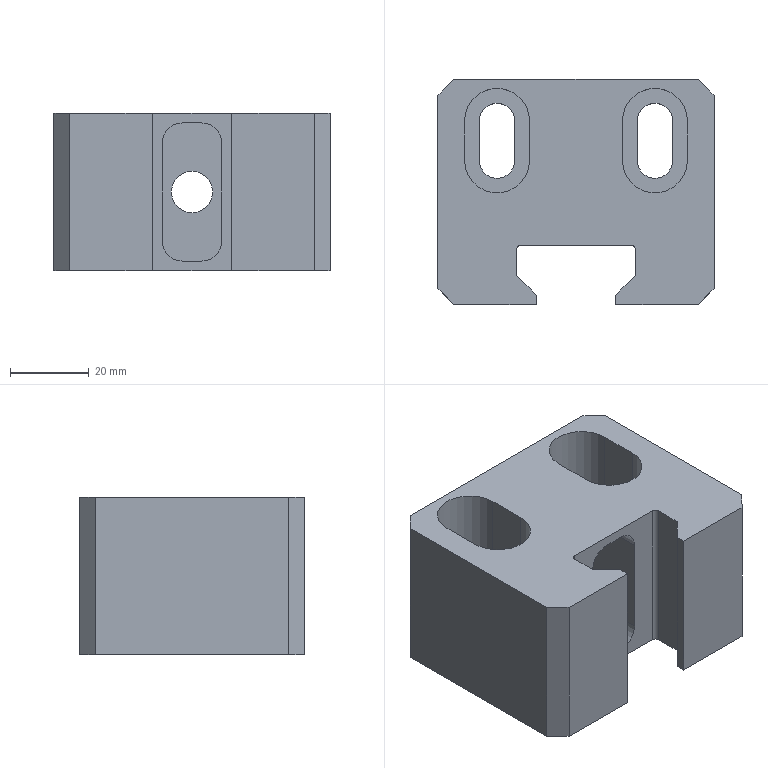Part | SolidWorks | features BaseBody 1 | 1 solid | 49 faces | box 70 x 57 x 40 mm | volume 110609 mm3 | plane 33 | cylinder 16 | commonest cylinder face diameters 9 x4 10 x4 16.5 x4 2 x2 10.5 x2
STEP:
#1=CARTESIAN_POINT('',(0.,16.,-25.25));
#2=VERTEX_POINT('',#1);
#3=CARTESIAN_POINT('',(0.,16.,-14.75));
#4=VERTEX_POINT('',#3);
#5=CARTESIAN_POINT('',(0.,16.,-20.));
#6=DIRECTION('',(0.,1.,0.));
#7=DIRECTION('',(0.,0.,1.));
#8=AXIS2_PLACEMENT_3D('',#5,#6,#7);
#9=CIRCLE('',#8,5.25);
#10=EDGE_CURVE('',#2,#4,#9,.T.);
#11=ORIENTED_EDGE('',*,*,#10,.F.);
#12=CARTESIAN_POINT('',(0.,42.,-25.25));
#13=VERTEX_POINT('',#12);
#14=CARTESIAN_POINT('',(0.,42.,-25.25));
#15=DIRECTION('',(0.,1.,0.));
#16=VECTOR('',#15,1000.);
#17=LINE('',#14,#16);
#18=EDGE_CURVE('',#2,#13,#17,.T.);
#19=ORIENTED_EDGE('',*,*,#18,.T.);
#20=CARTESIAN_POINT('',(0.,42.,-14.75));
#21=VERTEX_POINT('',#20);
#22=CARTESIAN_POINT('',(0.,42.,-20.));
#23=DIRECTION('',(0.,-1.,0.));
#24=DIRECTION('',(0.,0.,1.));
#25=AXIS2_PLACEMENT_3D('',#22,#23,#24);
#26=CIRCLE('',#25,5.25);
#27=EDGE_CURVE('',#21,#13,#26,.T.);
#28=ORIENTED_EDGE('',*,*,#27,.F.);
#29=CARTESIAN_POINT('',(0.,42.,-14.75));
#30=DIRECTION('',(0.,1.,0.));
#31=VECTOR('',#30,1000.);
#32=LINE('',#29,#31);
#33=EDGE_CURVE('',#4,#21,#32,.T.);
#34=ORIENTED_EDGE('',*,*,#33,.F.);
#35=EDGE_LOOP('',(#11,#19,#28,#34));
#36=FACE_OUTER_BOUND('',#35,.T.);
#37=CARTESIAN_POINT('',(0.,42.,-20.));
#38=DIRECTION('',(0.,1.,0.));
#39=DIRECTION('',(0.,0.,1.));
#40=AXIS2_PLACEMENT_3D('',#37,#38,#39);
#41=CYLINDRICAL_SURFACE('',#40,5.25);
#42=ADVANCED_FACE('',(#36),#41,.F.);
#43=CARTESIAN_POINT('',(-35.,-11.,-40.));
#44=VERTEX_POINT('',#43);
#45=CARTESIAN_POINT('',(-31.,-15.,-40.));
#46=VERTEX_POINT('',#45);
#47=CARTESIAN_POINT('',(-35.,-11.,-40.));
#48=DIRECTION('',(0.7071,-0.7071,0.));
#49=VECTOR('',#48,1000.);
#50=LINE('',#47,#49);
#51=EDGE_CURVE('',#44,#46,#50,.T.);
#52=ORIENTED_EDGE('',*,*,#51,.F.);
#53=CARTESIAN_POINT('',(-35.,38.,-40.));
#54=VERTEX_POINT('',#53);
#55=CARTESIAN_POINT('',(-35.,0.,-40.));
#56=DIRECTION('',(0.,-1.,0.));
#57=VECTOR('',#56,1000.);
#58=LINE('',#55,#57);
#59=EDGE_CURVE('',#54,#44,#58,.T.);
#60=ORIENTED_EDGE('',*,*,#59,.F.);
#61=CARTESIAN_POINT('',(-31.,42.,-40.));
#62=VERTEX_POINT('',#61);
#63=CARTESIAN_POINT('',(-31.,42.,-40.));
#64=DIRECTION('',(-0.7071,-0.7071,0.));
#65=VECTOR('',#64,1000.);
#66=LINE('',#63,#65);
#67=EDGE_CURVE('',#62,#54,#66,.T.);
#68=ORIENTED_EDGE('',*,*,#67,.F.);
#69=CARTESIAN_POINT('',(31.,42.,-40.));
#70=VERTEX_POINT('',#69);
#71=CARTESIAN_POINT('',(0.,42.,-40.));
#72=DIRECTION('',(-1.,0.,0.));
#73=VECTOR('',#72,1000.);
#74=LINE('',#71,#73);
#75=EDGE_CURVE('',#70,#62,#74,.T.);
#76=ORIENTED_EDGE('',*,*,#75,.F.);
#77=CARTESIAN_POINT('',(35.,38.,-40.));
#78=VERTEX_POINT('',#77);
#79=CARTESIAN_POINT('',(35.,38.,-40.));
#80=DIRECTION('',(-0.7071,0.7071,0.));
#81=VECTOR('',#80,1000.);
#82=LINE('',#79,#81);
#83=EDGE_CURVE('',#78,#70,#82,.T.);
#84=ORIENTED_EDGE('',*,*,#83,.F.);
#85=CARTESIAN_POINT('',(35.,-11.,-40.));
#86=VERTEX_POINT('',#85);
#87=CARTESIAN_POINT('',(35.,0.,-40.));
#88=DIRECTION('',(0.,1.,0.));
#89=VECTOR('',#88,1000.);
#90=LINE('',#87,#89);
#91=EDGE_CURVE('',#86,#78,#90,.T.);
#92=ORIENTED_EDGE('',*,*,#91,.F.);
#93=CARTESIAN_POINT('',(31.,-15.,-40.));
#94=VERTEX_POINT('',#93);
#95=CARTESIAN_POINT('',(31.,-15.,-40.));
#96=DIRECTION('',(0.7071,0.7071,0.));
#97=VECTOR('',#96,1000.);
#98=LINE('',#95,#97);
#99=EDGE_CURVE('',#94,#86,#98,.T.);
#100=ORIENTED_EDGE('',*,*,#99,.F.);
#101=CARTESIAN_POINT('',(10.1,-15.,-40.));
#102=VERTEX_POINT('',#101);
#103=CARTESIAN_POINT('',(0.,-15.,-40.));
#104=DIRECTION('',(1.,0.,0.));
#105=VECTOR('',#104,1000.);
#106=LINE('',#103,#105);
#107=EDGE_CURVE('',#102,#94,#106,.T.);
#108=ORIENTED_EDGE('',*,*,#107,.F.);
#109=CARTESIAN_POINT('',(10.1,-12.662,-40.));
#110=VERTEX_POINT('',#109);
#111=CARTESIAN_POINT('',(10.1,0.,-40.));
#112=DIRECTION('',(0.,-1.,0.));
#113=VECTOR('',#112,1000.);
#114=LINE('',#111,#113);
#115=EDGE_CURVE('',#110,#102,#114,.T.);
#116=ORIENTED_EDGE('',*,*,#115,.F.);
#117=CARTESIAN_POINT('',(15.,-7.762,-40.));
#118=VERTEX_POINT('',#117);
#119=CARTESIAN_POINT('',(15.,-7.762,-40.));
#120=DIRECTION('',(-0.7071,-0.7071,0.));
#121=VECTOR('',#120,1000.);
#122=LINE('',#119,#121);
#123=EDGE_CURVE('',#118,#110,#122,.T.);
#124=ORIENTED_EDGE('',*,*,#123,.F.);
#125=CARTESIAN_POINT('',(15.,-1.,-40.));
#126=VERTEX_POINT('',#125);
#127=CARTESIAN_POINT('',(15.,0.,-40.));
#128=DIRECTION('',(0.,-1.,0.));
#129=VECTOR('',#128,1000.);
#130=LINE('',#127,#129);
#131=EDGE_CURVE('',#126,#118,#130,.T.);
#132=ORIENTED_EDGE('',*,*,#131,.F.);
#133=CARTESIAN_POINT('',(14.,0.,-40.));
#134=VERTEX_POINT('',#133);
#135=CARTESIAN_POINT('',(14.,-1.,-40.));
#136=DIRECTION('',(0.,0.,1.));
#137=DIRECTION('',(-1.,0.,0.));
#138=AXIS2_PLACEMENT_3D('',#135,#136,#137);
#139=CIRCLE('',#138,1.);
#140=EDGE_CURVE('',#126,#134,#139,.T.);
#141=ORIENTED_EDGE('',*,*,#140,.T.);
#142=CARTESIAN_POINT('',(-14.,0.,-40.));
#143=VERTEX_POINT('',#142);
#144=CARTESIAN_POINT('',(0.,0.,-40.));
#145=DIRECTION('',(1.,0.,0.));
#146=VECTOR('',#145,1000.);
#147=LINE('',#144,#146);
#148=EDGE_CURVE('',#143,#134,#147,.T.);
#149=ORIENTED_EDGE('',*,*,#148,.F.);
#150=CARTESIAN_POINT('',(-15.,-1.,-40.));
#151=VERTEX_POINT('',#150);
#152=CARTESIAN_POINT('',(-14.,-1.,-40.));
#153=DIRECTION('',(0.,0.,1.));
#154=DIRECTION('',(-1.,0.,0.));
#155=AXIS2_PLACEMENT_3D('',#152,#153,#154);
#156=CIRCLE('',#155,1.);
#157=EDGE_CURVE('',#143,#151,#156,.T.);
#158=ORIENTED_EDGE('',*,*,#157,.T.);
#159=CARTESIAN_POINT('',(-15.,-7.762,-40.));
#160=VERTEX_POINT('',#159);
#161=CARTESIAN_POINT('',(-15.,0.,-40.));
#162=DIRECTION('',(0.,1.,0.));
#163=VECTOR('',#162,1000.);
#164=LINE('',#161,#163);
#165=EDGE_CURVE('',#160,#151,#164,.T.);
#166=ORIENTED_EDGE('',*,*,#165,.F.);
#167=CARTESIAN_POINT('',(-10.1,-12.662,-40.));
#168=VERTEX_POINT('',#167);
#169=CARTESIAN_POINT('',(-10.1,-12.662,-40.));
#170=DIRECTION('',(-0.7071,0.7071,0.));
#171=VECTOR('',#170,1000.);
#172=LINE('',#169,#171);
#173=EDGE_CURVE('',#168,#160,#172,.T.);
#174=ORIENTED_EDGE('',*,*,#173,.F.);
#175=CARTESIAN_POINT('',(-10.1,-15.,-40.));
#176=VERTEX_POINT('',#175);
#177=CARTESIAN_POINT('',(-10.1,0.,-40.));
#178=DIRECTION('',(0.,1.,0.));
#179=VECTOR('',#178,1000.);
#180=LINE('',#177,#179);
#181=EDGE_CURVE('',#176,#168,#180,.T.);
#182=ORIENTED_EDGE('',*,*,#181,.F.);
#183=CARTESIAN_POINT('',(0.,-15.,-40.));
#184=DIRECTION('',(1.,0.,0.));
#185=VECTOR('',#184,1000.);
#186=LINE('',#183,#185);
#187=EDGE_CURVE('',#46,#176,#186,.T.);
#188=ORIENTED_EDGE('',*,*,#187,.F.);
#189=EDGE_LOOP('',(#52,#60,#68,#76,#84,#92,#100,#108,#116,#124,#132,#141,#149,#158,#166,#174,#182,#188));
#190=FACE_OUTER_BOUND('',#189,.T.);
#191=CARTESIAN_POINT('',(-15.5,21.5,-40.));
#192=VERTEX_POINT('',#191);
#193=CARTESIAN_POINT('',(-24.5,21.5,-40.));
#194=VERTEX_POINT('',#193);
#195=CARTESIAN_POINT('',(-20.,21.5,-40.));
#196=DIRECTION('',(0.,0.,-1.));
#197=DIRECTION('',(1.,0.,0.));
#198=AXIS2_PLACEMENT_3D('',#195,#196,#197);
#199=CIRCLE('',#198,4.5);
#200=EDGE_CURVE('',#192,#194,#199,.T.);
#201=ORIENTED_EDGE('',*,*,#200,.F.);
#202=CARTESIAN_POINT('',(-15.5,31.5,-40.));
#203=VERTEX_POINT('',#202);
#204=CARTESIAN_POINT('',(-15.5,0.,-40.));
#205=DIRECTION('',(0.,-1.,0.));
#206=VECTOR('',#205,1000.);
#207=LINE('',#204,#206);
#208=EDGE_CURVE('',#203,#192,#207,.T.);
#209=ORIENTED_EDGE('',*,*,#208,.F.);
#210=CARTESIAN_POINT('',(-24.5,31.5,-40.));
#211=VERTEX_POINT('',#210);
#212=CARTESIAN_POINT('',(-20.,31.5,-40.));
#213=DIRECTION('',(0.,0.,-1.));
#214=DIRECTION('',(1.,0.,0.));
#215=AXIS2_PLACEMENT_3D('',#212,#213,#214);
#216=CIRCLE('',#215,4.5);
#217=EDGE_CURVE('',#211,#203,#216,.T.);
#218=ORIENTED_EDGE('',*,*,#217,.F.);
#219=CARTESIAN_POINT('',(-24.5,0.,-40.));
#220=DIRECTION('',(0.,1.,0.));
#221=VECTOR('',#220,1000.);
#222=LINE('',#219,#221);
#223=EDGE_CURVE('',#194,#211,#222,.T.);
#224=ORIENTED_EDGE('',*,*,#223,.F.);
#225=EDGE_LOOP('',(#201,#209,#218,#224));
#226=FACE_BOUND('',#225,.T.);
#227=CARTESIAN_POINT('',(15.5,31.5,-40.));
#228=VERTEX_POINT('',#227);
#229=CARTESIAN_POINT('',(24.5,31.5,-40.));
#230=VERTEX_POINT('',#229);
#231=CARTESIAN_POINT('',(20.,31.5,-40.));
#232=DIRECTION('',(0.,0.,-1.));
#233=DIRECTION('',(1.,0.,0.));
#234=AXIS2_PLACEMENT_3D('',#231,#232,#233);
#235=CIRCLE('',#234,4.5);
#236=EDGE_CURVE('',#228,#230,#235,.T.);
#237=ORIENTED_EDGE('',*,*,#236,.F.);
#238=CARTESIAN_POINT('',(15.5,21.5,-40.));
#239=VERTEX_POINT('',#238);
#240=CARTESIAN_POINT('',(15.5,0.,-40.));
#241=DIRECTION('',(0.,1.,0.));
#242=VECTOR('',#241,1000.);
#243=LINE('',#240,#242);
#244=EDGE_CURVE('',#239,#228,#243,.T.);
#245=ORIENTED_EDGE('',*,*,#244,.F.);
#246=CARTESIAN_POINT('',(24.5,21.5,-40.));
#247=VERTEX_POINT('',#246);
#248=CARTESIAN_POINT('',(20.,21.5,-40.));
#249=DIRECTION('',(0.,0.,-1.));
#250=DIRECTION('',(1.,0.,0.));
#251=AXIS2_PLACEMENT_3D('',#248,#249,#250);
#252=CIRCLE('',#251,4.5);
#253=EDGE_CURVE('',#247,#239,#252,.T.);
#254=ORIENTED_EDGE('',*,*,#253,.F.);
#255=CARTESIAN_POINT('',(24.5,0.,-40.));
#256=DIRECTION('',(0.,-1.,0.));
#257=VECTOR('',#256,1000.);
#258=LINE('',#255,#257);
#259=EDGE_CURVE('',#230,#247,#258,.T.);
#260=ORIENTED_EDGE('',*,*,#259,.F.);
#261=EDGE_LOOP('',(#237,#245,#254,#260));
#262=FACE_BOUND('',#261,.T.);
#263=CARTESIAN_POINT('',(0.,0.,-40.));
#264=DIRECTION('',(0.,0.,1.));
#265=DIRECTION('',(1.,0.,0.));
#266=AXIS2_PLACEMENT_3D('',#263,#264,#265);
#267=PLANE('',#266);
#268=ADVANCED_FACE('',(#190,#226,#262),#267,.F.);
#269=ORIENTED_EDGE('',*,*,#187,.T.);
#270=CARTESIAN_POINT('',(-10.1,-15.,0.));
#271=VERTEX_POINT('',#270);
#272=CARTESIAN_POINT('',(-10.1,-15.,-40.));
#273=DIRECTION('',(0.,0.,1.));
#274=VECTOR('',#273,1000.);
#275=LINE('',#272,#274);
#276=EDGE_CURVE('',#176,#271,#275,.T.);
#277=ORIENTED_EDGE('',*,*,#276,.T.);
#278=CARTESIAN_POINT('',(-31.,-15.,0.));
#279=VERTEX_POINT('',#278);
#280=CARTESIAN_POINT('',(-10.1,-15.,0.));
#281=DIRECTION('',(-1.,0.,0.));
#282=VECTOR('',#281,1000.);
#283=LINE('',#280,#282);
#284=EDGE_CURVE('',#271,#279,#283,.T.);
#285=ORIENTED_EDGE('',*,*,#284,.T.);
#286=CARTESIAN_POINT('',(-31.,-15.,-40.));
#287=DIRECTION('',(0.,0.,-1.));
#288=VECTOR('',#287,1000.);
#289=LINE('',#286,#288);
#290=EDGE_CURVE('',#279,#46,#289,.T.);
#291=ORIENTED_EDGE('',*,*,#290,.T.);
#292=EDGE_LOOP('',(#269,#277,#285,#291));
#293=FACE_OUTER_BOUND('',#292,.T.);
#294=CARTESIAN_POINT('',(-10.1,-15.,-40.));
#295=DIRECTION('',(0.,-1.,0.));
#296=DIRECTION('',(1.,0.,0.));
#297=AXIS2_PLACEMENT_3D('',#294,#295,#296);
#298=PLANE('',#297);
#299=ADVANCED_FACE('',(#293),#298,.T.);
#300=ORIENTED_EDGE('',*,*,#290,.F.);
#301=CARTESIAN_POINT('',(-35.,-11.,0.));
#302=VERTEX_POINT('',#301);
#303=CARTESIAN_POINT('',(-35.,-11.,0.));
#304=DIRECTION('',(0.7071,-0.7071,0.));
#305=VECTOR('',#304,1000.);
#306=LINE('',#303,#305);
#307=EDGE_CURVE('',#302,#279,#306,.T.);
#308=ORIENTED_EDGE('',*,*,#307,.F.);
#309=CARTESIAN_POINT('',(-35.,-11.,-40.));
#310=DIRECTION('',(0.,0.,1.));
#311=VECTOR('',#310,1000.);
#312=LINE('',#309,#311);
#313=EDGE_CURVE('',#44,#302,#312,.T.);
#314=ORIENTED_EDGE('',*,*,#313,.F.);
#315=ORIENTED_EDGE('',*,*,#51,.T.);
#316=EDGE_LOOP('',(#300,#308,#314,#315));
#317=FACE_OUTER_BOUND('',#316,.T.);
#318=CARTESIAN_POINT('',(-35.,-11.,-40.));
#319=DIRECTION('',(0.7071,0.7071,0.));
#320=DIRECTION('',(-0.7071,0.7071,0.));
#321=AXIS2_PLACEMENT_3D('',#318,#319,#320);
#322=PLANE('',#321);
#323=ADVANCED_FACE('',(#317),#322,.F.);
#324=CARTESIAN_POINT('',(-35.,38.,0.));
#325=VERTEX_POINT('',#324);
#326=CARTESIAN_POINT('',(-35.,42.,0.));
#327=DIRECTION('',(0.,1.,0.));
#328=VECTOR('',#327,1000.);
#329=LINE('',#326,#328);
#330=EDGE_CURVE('',#302,#325,#329,.T.);
#331=ORIENTED_EDGE('',*,*,#330,.T.);
#332=CARTESIAN_POINT('',(-35.,38.,-40.));
#333=DIRECTION('',(0.,0.,-1.));
#334=VECTOR('',#333,1000.);
#335=LINE('',#332,#334);
#336=EDGE_CURVE('',#325,#54,#335,.T.);
#337=ORIENTED_EDGE('',*,*,#336,.T.);
#338=ORIENTED_EDGE('',*,*,#59,.T.);
#339=ORIENTED_EDGE('',*,*,#313,.T.);
#340=EDGE_LOOP('',(#331,#337,#338,#339));
#341=FACE_OUTER_BOUND('',#340,.T.);
#342=CARTESIAN_POINT('',(-35.,42.,-40.));
#343=DIRECTION('',(-1.,0.,0.));
#344=DIRECTION('',(0.,-1.,0.));
#345=AXIS2_PLACEMENT_3D('',#342,#343,#344);
#346=PLANE('',#345);
#347=ADVANCED_FACE('',(#341),#346,.T.);
#348=ORIENTED_EDGE('',*,*,#336,.F.);
#349=CARTESIAN_POINT('',(-31.,42.,0.));
#350=VERTEX_POINT('',#349);
#351=CARTESIAN_POINT('',(-31.,42.,0.));
#352=DIRECTION('',(-0.7071,-0.7071,0.));
#353=VECTOR('',#352,1000.);
#354=LINE('',#351,#353);
#355=EDGE_CURVE('',#350,#325,#354,.T.);
#356=ORIENTED_EDGE('',*,*,#355,.F.);
#357=CARTESIAN_POINT('',(-31.,42.,-40.));
#358=DIRECTION('',(0.,0.,1.));
#359=VECTOR('',#358,1000.);
#360=LINE('',#357,#359);
#361=EDGE_CURVE('',#62,#350,#360,.T.);
#362=ORIENTED_EDGE('',*,*,#361,.F.);
#363=ORIENTED_EDGE('',*,*,#67,.T.);
#364=EDGE_LOOP('',(#348,#356,#362,#363));
#365=FACE_OUTER_BOUND('',#364,.T.);
#366=CARTESIAN_POINT('',(-31.,42.,-40.));
#367=DIRECTION('',(0.7071,-0.7071,0.));
#368=DIRECTION('',(0.7071,0.7071,0.));
#369=AXIS2_PLACEMENT_3D('',#366,#367,#368);
#370=PLANE('',#369);
#371=ADVANCED_FACE('',(#365),#370,.F.);
#372=ORIENTED_EDGE('',*,*,#75,.T.);
#373=ORIENTED_EDGE('',*,*,#361,.T.);
#374=CARTESIAN_POINT('',(31.,42.,0.));
#375=VERTEX_POINT('',#374);
#376=CARTESIAN_POINT('',(35.,42.,0.));
#377=DIRECTION('',(1.,0.,0.));
#378=VECTOR('',#377,1000.);
#379=LINE('',#376,#378);
#380=EDGE_CURVE('',#350,#375,#379,.T.);
#381=ORIENTED_EDGE('',*,*,#380,.T.);
#382=CARTESIAN_POINT('',(31.,42.,-40.));
#383=DIRECTION('',(0.,0.,-1.));
#384=VECTOR('',#383,1000.);
#385=LINE('',#382,#384);
#386=EDGE_CURVE('',#375,#70,#385,.T.);
#387=ORIENTED_EDGE('',*,*,#386,.T.);
#388=EDGE_LOOP('',(#372,#373,#381,#387));
#389=FACE_OUTER_BOUND('',#388,.T.);
#390=ORIENTED_EDGE('',*,*,#27,.T.);
#391=CARTESIAN_POINT('',(0.,42.,-20.));
#392=DIRECTION('',(0.,-1.,0.));
#393=DIRECTION('',(0.,0.,1.));
#394=AXIS2_PLACEMENT_3D('',#391,#392,#393);
#395=CIRCLE('',#394,5.25);
#396=EDGE_CURVE('',#13,#21,#395,.T.);
#397=ORIENTED_EDGE('',*,*,#396,.T.);
#398=EDGE_LOOP('',(#390,#397));
#399=FACE_BOUND('',#398,.T.);
#400=CARTESIAN_POINT('',(35.,42.,-40.));
#401=DIRECTION('',(0.,1.,0.));
#402=DIRECTION('',(-1.,0.,0.));
#403=AXIS2_PLACEMENT_3D('',#400,#401,#402);
#404=PLANE('',#403);
#405=ADVANCED_FACE('',(#389,#399),#404,.T.);
#406=ORIENTED_EDGE('',*,*,#386,.F.);
#407=CARTESIAN_POINT('',(35.,38.,0.));
#408=VERTEX_POINT('',#407);
#409=CARTESIAN_POINT('',(35.,38.,0.));
#410=DIRECTION('',(-0.7071,0.7071,0.));
#411=VECTOR('',#410,1000.);
#412=LINE('',#409,#411);
#413=EDGE_CURVE('',#408,#375,#412,.T.);
#414=ORIENTED_EDGE('',*,*,#413,.F.);
#415=CARTESIAN_POINT('',(35.,38.,-40.));
#416=DIRECTION('',(0.,0.,1.));
#417=VECTOR('',#416,1000.);
#418=LINE('',#415,#417);
#419=EDGE_CURVE('',#78,#408,#418,.T.);
#420=ORIENTED_EDGE('',*,*,#419,.F.);
#421=ORIENTED_EDGE('',*,*,#83,.T.);
#422=EDGE_LOOP('',(#406,#414,#420,#421));
#423=FACE_OUTER_BOUND('',#422,.T.);
#424=CARTESIAN_POINT('',(35.,38.,-40.));
#425=DIRECTION('',(-0.7071,-0.7071,0.));
#426=DIRECTION('',(0.7071,-0.7071,0.));
#427=AXIS2_PLACEMENT_3D('',#424,#425,#426);
#428=PLANE('',#427);
#429=ADVANCED_FACE('',(#423),#428,.F.);
#430=ORIENTED_EDGE('',*,*,#91,.T.);
#431=ORIENTED_EDGE('',*,*,#419,.T.);
#432=CARTESIAN_POINT('',(35.,-11.,0.));
#433=VERTEX_POINT('',#432);
#434=CARTESIAN_POINT('',(35.,42.,0.));
#435=DIRECTION('',(0.,-1.,0.));
#436=VECTOR('',#435,1000.);
#437=LINE('',#434,#436);
#438=EDGE_CURVE('',#408,#433,#437,.T.);
#439=ORIENTED_EDGE('',*,*,#438,.T.);
#440=CARTESIAN_POINT('',(35.,-11.,-40.));
#441=DIRECTION('',(0.,0.,-1.));
#442=VECTOR('',#441,1000.);
#443=LINE('',#440,#442);
#444=EDGE_CURVE('',#433,#86,#443,.T.);
#445=ORIENTED_EDGE('',*,*,#444,.T.);
#446=EDGE_LOOP('',(#430,#431,#439,#445));
#447=FACE_OUTER_BOUND('',#446,.T.);
#448=CARTESIAN_POINT('',(35.,42.,-40.));
#449=DIRECTION('',(1.,0.,0.));
#450=DIRECTION('',(0.,1.,0.));
#451=AXIS2_PLACEMENT_3D('',#448,#449,#450);
#452=PLANE('',#451);
#453=ADVANCED_FACE('',(#447),#452,.T.);
#454=ORIENTED_EDGE('',*,*,#444,.F.);
#455=CARTESIAN_POINT('',(31.,-15.,0.));
#456=VERTEX_POINT('',#455);
#457=CARTESIAN_POINT('',(31.,-15.,0.));
#458=DIRECTION('',(0.7071,0.7071,0.));
#459=VECTOR('',#458,1000.);
#460=LINE('',#457,#459);
#461=EDGE_CURVE('',#456,#433,#460,.T.);
#462=ORIENTED_EDGE('',*,*,#461,.F.);
#463=CARTESIAN_POINT('',(31.,-15.,-40.));
#464=DIRECTION('',(0.,0.,1.));
#465=VECTOR('',#464,1000.);
#466=LINE('',#463,#465);
#467=EDGE_CURVE('',#94,#456,#466,.T.);
#468=ORIENTED_EDGE('',*,*,#467,.F.);
#469=ORIENTED_EDGE('',*,*,#99,.T.);
#470=EDGE_LOOP('',(#454,#462,#468,#469));
#471=FACE_OUTER_BOUND('',#470,.T.);
#472=CARTESIAN_POINT('',(31.,-15.,-40.));
#473=DIRECTION('',(-0.7071,0.7071,0.));
#474=DIRECTION('',(-0.7071,-0.7071,0.));
#475=AXIS2_PLACEMENT_3D('',#472,#473,#474);
#476=PLANE('',#475);
#477=ADVANCED_FACE('',(#471),#476,.F.);
#478=CARTESIAN_POINT('',(10.1,-15.,0.));
#479=VERTEX_POINT('',#478);
#480=CARTESIAN_POINT('',(10.1,-15.,0.));
#481=DIRECTION('',(-1.,0.,0.));
#482=VECTOR('',#481,1000.);
#483=LINE('',#480,#482);
#484=EDGE_CURVE('',#456,#479,#483,.T.);
#485=ORIENTED_EDGE('',*,*,#484,.T.);
#486=CARTESIAN_POINT('',(10.1,-15.,-40.));
#487=DIRECTION('',(0.,0.,-1.));
#488=VECTOR('',#487,1000.);
#489=LINE('',#486,#488);
#490=EDGE_CURVE('',#479,#102,#489,.T.);
#491=ORIENTED_EDGE('',*,*,#490,.T.);
#492=ORIENTED_EDGE('',*,*,#107,.T.);
#493=ORIENTED_EDGE('',*,*,#467,.T.);
#494=EDGE_LOOP('',(#485,#491,#492,#493));
#495=FACE_OUTER_BOUND('',#494,.T.);
#496=CARTESIAN_POINT('',(10.1,-15.,-40.));
#497=DIRECTION('',(0.,-1.,0.));
#498=DIRECTION('',(1.,0.,0.));
#499=AXIS2_PLACEMENT_3D('',#496,#497,#498);
#500=PLANE('',#499);
#501=ADVANCED_FACE('',(#495),#500,.T.);
#502=ORIENTED_EDGE('',*,*,#115,.T.);
#503=ORIENTED_EDGE('',*,*,#490,.F.);
#504=CARTESIAN_POINT('',(10.1,-12.662,0.));
#505=VERTEX_POINT('',#504);
#506=CARTESIAN_POINT('',(10.1,-15.,0.));
#507=DIRECTION('',(0.,1.,0.));
#508=VECTOR('',#507,1000.);
#509=LINE('',#506,#508);
#510=EDGE_CURVE('',#479,#505,#509,.T.);
#511=ORIENTED_EDGE('',*,*,#510,.T.);
#512=CARTESIAN_POINT('',(10.1,-12.662,-40.));
#513=DIRECTION('',(0.,0.,-1.));
#514=VECTOR('',#513,1000.);
#515=LINE('',#512,#514);
#516=EDGE_CURVE('',#505,#110,#515,.T.);
#517=ORIENTED_EDGE('',*,*,#516,.T.);
#518=EDGE_LOOP('',(#502,#503,#511,#517));
#519=FACE_OUTER_BOUND('',#518,.T.);
#520=CARTESIAN_POINT('',(10.1,-15.,-40.));
#521=DIRECTION('',(-1.,0.,0.));
#522=DIRECTION('',(0.,-1.,0.));
#523=AXIS2_PLACEMENT_3D('',#520,#521,#522);
#524=PLANE('',#523);
#525=ADVANCED_FACE('',(#519),#524,.T.);
#526=ORIENTED_EDGE('',*,*,#123,.T.);
#527=ORIENTED_EDGE('',*,*,#516,.F.);
#528=CARTESIAN_POINT('',(15.,-7.762,0.));
#529=VERTEX_POINT('',#528);
#530=CARTESIAN_POINT('',(10.1,-12.662,0.));
#531=DIRECTION('',(0.7071,0.7071,0.));
#532=VECTOR('',#531,1000.);
#533=LINE('',#530,#532);
#534=EDGE_CURVE('',#505,#529,#533,.T.);
#535=ORIENTED_EDGE('',*,*,#534,.T.);
#536=CARTESIAN_POINT('',(15.,-7.762,-40.));
#537=DIRECTION('',(0.,0.,-1.));
#538=VECTOR('',#537,1000.);
#539=LINE('',#536,#538);
#540=EDGE_CURVE('',#529,#118,#539,.T.);
#541=ORIENTED_EDGE('',*,*,#540,.T.);
#542=EDGE_LOOP('',(#526,#527,#535,#541));
#543=FACE_OUTER_BOUND('',#542,.T.);
#544=CARTESIAN_POINT('',(10.1,-12.662,-40.));
#545=DIRECTION('',(-0.7071,0.7071,0.));
#546=DIRECTION('',(-0.7071,-0.7071,0.));
#547=AXIS2_PLACEMENT_3D('',#544,#545,#546);
#548=PLANE('',#547);
#549=ADVANCED_FACE('',(#543),#548,.T.);
#550=ORIENTED_EDGE('',*,*,#131,.T.);
#551=ORIENTED_EDGE('',*,*,#540,.F.);
#552=CARTESIAN_POINT('',(15.,-1.,0.));
#553=VERTEX_POINT('',#552);
#554=CARTESIAN_POINT('',(15.,0.,0.));
#555=DIRECTION('',(0.,1.,0.));
#556=VECTOR('',#555,1000.);
#557=LINE('',#554,#556);
#558=EDGE_CURVE('',#529,#553,#557,.T.);
#559=ORIENTED_EDGE('',*,*,#558,.T.);
#560=CARTESIAN_POINT('',(15.,-1.,-40.));
#561=DIRECTION('',(0.,0.,-1.));
#562=VECTOR('',#561,1000.);
#563=LINE('',#560,#562);
#564=EDGE_CURVE('',#553,#126,#563,.T.);
#565=ORIENTED_EDGE('',*,*,#564,.T.);
#566=EDGE_LOOP('',(#550,#551,#559,#565));
#567=FACE_OUTER_BOUND('',#566,.T.);
#568=CARTESIAN_POINT('',(15.,0.,-40.));
#569=DIRECTION('',(-1.,0.,0.));
#570=DIRECTION('',(0.,0.,1.));
#571=AXIS2_PLACEMENT_3D('',#568,#569,#570);
#572=PLANE('',#571);
#573=ADVANCED_FACE('',(#567),#572,.T.);
#574=CARTESIAN_POINT('',(14.,0.,0.));
#575=VERTEX_POINT('',#574);
#576=CARTESIAN_POINT('',(-14.,0.,0.));
#577=VERTEX_POINT('',#576);
#578=CARTESIAN_POINT('',(15.,0.,0.));
#579=DIRECTION('',(-1.,0.,0.));
#580=VECTOR('',#579,1000.);
#581=LINE('',#578,#580);
#582=EDGE_CURVE('',#575,#577,#581,.T.);
#583=ORIENTED_EDGE('',*,*,#582,.T.);
#584=CARTESIAN_POINT('',(-14.,0.,-40.));
#585=DIRECTION('',(0.,0.,-1.));
#586=VECTOR('',#585,1000.);
#587=LINE('',#584,#586);
#588=EDGE_CURVE('',#577,#143,#587,.T.);
#589=ORIENTED_EDGE('',*,*,#588,.T.);
#590=ORIENTED_EDGE('',*,*,#148,.T.);
#591=CARTESIAN_POINT('',(14.,0.,-40.));
#592=DIRECTION('',(0.,0.,1.));
#593=VECTOR('',#592,1000.);
#594=LINE('',#591,#593);
#595=EDGE_CURVE('',#134,#575,#594,.T.);
#596=ORIENTED_EDGE('',*,*,#595,.T.);
#597=EDGE_LOOP('',(#583,#589,#590,#596));
#598=FACE_OUTER_BOUND('',#597,.T.);
#599=CARTESIAN_POINT('',(-2.5,0.,-2.5));
#600=VERTEX_POINT('',#599);
#601=CARTESIAN_POINT('',(2.5,0.,-2.5));
#602=VERTEX_POINT('',#601);
#603=CARTESIAN_POINT('',(15.,0.,-2.5));
#604=DIRECTION('',(1.,0.,0.));
#605=VECTOR('',#604,1000.);
#606=LINE('',#603,#605);
#607=EDGE_CURVE('',#600,#602,#606,.T.);
#608=ORIENTED_EDGE('',*,*,#607,.T.);
#609=CARTESIAN_POINT('',(7.5,0.,-7.5));
#610=VERTEX_POINT('',#609);
#611=CARTESIAN_POINT('',(2.5,0.,-7.5));
#612=DIRECTION('',(0.,1.,0.));
#613=DIRECTION('',(0.,0.,1.));
#614=AXIS2_PLACEMENT_3D('',#611,#612,#613);
#615=CIRCLE('',#614,5.);
#616=EDGE_CURVE('',#602,#610,#615,.T.);
#617=ORIENTED_EDGE('',*,*,#616,.T.);
#618=CARTESIAN_POINT('',(7.5,0.,-32.5));
#619=VERTEX_POINT('',#618);
#620=CARTESIAN_POINT('',(7.5,0.,-40.));
#621=DIRECTION('',(0.,0.,-1.));
#622=VECTOR('',#621,1000.);
#623=LINE('',#620,#622);
#624=EDGE_CURVE('',#610,#619,#623,.T.);
#625=ORIENTED_EDGE('',*,*,#624,.T.);
#626=CARTESIAN_POINT('',(2.5,0.,-37.5));
#627=VERTEX_POINT('',#626);
#628=CARTESIAN_POINT('',(2.5,0.,-32.5));
#629=DIRECTION('',(0.,1.,0.));
#630=DIRECTION('',(0.,0.,1.));
#631=AXIS2_PLACEMENT_3D('',#628,#629,#630);
#632=CIRCLE('',#631,5.);
#633=EDGE_CURVE('',#619,#627,#632,.T.);
#634=ORIENTED_EDGE('',*,*,#633,.T.);
#635=CARTESIAN_POINT('',(-2.5,0.,-37.5));
#636=VERTEX_POINT('',#635);
#637=CARTESIAN_POINT('',(15.,0.,-37.5));
#638=DIRECTION('',(-1.,0.,0.));
#639=VECTOR('',#638,1000.);
#640=LINE('',#637,#639);
#641=EDGE_CURVE('',#627,#636,#640,.T.);
#642=ORIENTED_EDGE('',*,*,#641,.T.);
#643=CARTESIAN_POINT('',(-7.5,0.,-32.5));
#644=VERTEX_POINT('',#643);
#645=CARTESIAN_POINT('',(-2.5,0.,-32.5));
#646=DIRECTION('',(0.,1.,0.));
#647=DIRECTION('',(0.,0.,1.));
#648=AXIS2_PLACEMENT_3D('',#645,#646,#647);
#649=CIRCLE('',#648,5.);
#650=EDGE_CURVE('',#636,#644,#649,.T.);
#651=ORIENTED_EDGE('',*,*,#650,.T.);
#652=CARTESIAN_POINT('',(-7.5,0.,-7.5));
#653=VERTEX_POINT('',#652);
#654=CARTESIAN_POINT('',(-7.5,0.,-40.));
#655=DIRECTION('',(0.,0.,1.));
#656=VECTOR('',#655,1000.);
#657=LINE('',#654,#656);
#658=EDGE_CURVE('',#644,#653,#657,.T.);
#659=ORIENTED_EDGE('',*,*,#658,.T.);
#660=CARTESIAN_POINT('',(-2.5,0.,-7.5));
#661=DIRECTION('',(0.,1.,0.));
#662=DIRECTION('',(0.,0.,1.));
#663=AXIS2_PLACEMENT_3D('',#660,#661,#662);
#664=CIRCLE('',#663,5.);
#665=EDGE_CURVE('',#653,#600,#664,.T.);
#666=ORIENTED_EDGE('',*,*,#665,.T.);
#667=EDGE_LOOP('',(#608,#617,#625,#634,#642,#651,#659,#666));
#668=FACE_BOUND('',#667,.T.);
#669=CARTESIAN_POINT('',(15.,0.,-40.));
#670=DIRECTION('',(0.,-1.,0.));
#671=DIRECTION('',(1.,0.,0.));
#672=AXIS2_PLACEMENT_3D('',#669,#670,#671);
#673=PLANE('',#672);
#674=ADVANCED_FACE('',(#598,#668),#673,.T.);
#675=CARTESIAN_POINT('',(-15.,-1.,0.));
#676=VERTEX_POINT('',#675);
#677=CARTESIAN_POINT('',(-15.,-7.762,0.));
#678=VERTEX_POINT('',#677);
#679=CARTESIAN_POINT('',(-15.,0.,0.));
#680=DIRECTION('',(0.,-1.,0.));
#681=VECTOR('',#680,1000.);
#682=LINE('',#679,#681);
#683=EDGE_CURVE('',#676,#678,#682,.T.);
#684=ORIENTED_EDGE('',*,*,#683,.T.);
#685=CARTESIAN_POINT('',(-15.,-7.762,-40.));
#686=DIRECTION('',(0.,0.,-1.));
#687=VECTOR('',#686,1000.);
#688=LINE('',#685,#687);
#689=EDGE_CURVE('',#678,#160,#688,.T.);
#690=ORIENTED_EDGE('',*,*,#689,.T.);
#691=ORIENTED_EDGE('',*,*,#165,.T.);
#692=CARTESIAN_POINT('',(-15.,-1.,-40.));
#693=DIRECTION('',(0.,0.,1.));
#694=VECTOR('',#693,1000.);
#695=LINE('',#692,#694);
#696=EDGE_CURVE('',#151,#676,#695,.T.);
#697=ORIENTED_EDGE('',*,*,#696,.T.);
#698=EDGE_LOOP('',(#684,#690,#691,#697));
#699=FACE_OUTER_BOUND('',#698,.T.);
#700=CARTESIAN_POINT('',(-15.,0.,-40.));
#701=DIRECTION('',(1.,0.,0.));
#702=DIRECTION('',(0.,1.,0.));
#703=AXIS2_PLACEMENT_3D('',#700,#701,#702);
#704=PLANE('',#703);
#705=ADVANCED_FACE('',(#699),#704,.T.);
#706=ORIENTED_EDGE('',*,*,#173,.T.);
#707=ORIENTED_EDGE('',*,*,#689,.F.);
#708=CARTESIAN_POINT('',(-10.1,-12.662,0.));
#709=VERTEX_POINT('',#708);
#710=CARTESIAN_POINT('',(-15.,-7.762,0.));
#711=DIRECTION('',(0.7071,-0.7071,0.));
#712=VECTOR('',#711,1000.);
#713=LINE('',#710,#712);
#714=EDGE_CURVE('',#678,#709,#713,.T.);
#715=ORIENTED_EDGE('',*,*,#714,.T.);
#716=CARTESIAN_POINT('',(-10.1,-12.662,-40.));
#717=DIRECTION('',(0.,0.,-1.));
#718=VECTOR('',#717,1000.);
#719=LINE('',#716,#718);
#720=EDGE_CURVE('',#709,#168,#719,.T.);
#721=ORIENTED_EDGE('',*,*,#720,.T.);
#722=EDGE_LOOP('',(#706,#707,#715,#721));
#723=FACE_OUTER_BOUND('',#722,.T.);
#724=CARTESIAN_POINT('',(-15.,-7.762,-40.));
#725=DIRECTION('',(0.7071,0.7071,0.));
#726=DIRECTION('',(-0.7071,0.7071,0.));
#727=AXIS2_PLACEMENT_3D('',#724,#725,#726);
#728=PLANE('',#727);
#729=ADVANCED_FACE('',(#723),#728,.T.);
#730=ORIENTED_EDGE('',*,*,#181,.T.);
#731=ORIENTED_EDGE('',*,*,#720,.F.);
#732=CARTESIAN_POINT('',(-10.1,-15.,0.));
#733=DIRECTION('',(0.,-1.,0.));
#734=VECTOR('',#733,1000.);
#735=LINE('',#732,#734);
#736=EDGE_CURVE('',#709,#271,#735,.T.);
#737=ORIENTED_EDGE('',*,*,#736,.T.);
#738=ORIENTED_EDGE('',*,*,#276,.F.);
#739=EDGE_LOOP('',(#730,#731,#737,#738));
#740=FACE_OUTER_BOUND('',#739,.T.);
#741=CARTESIAN_POINT('',(-10.1,-15.,-40.));
#742=DIRECTION('',(1.,0.,0.));
#743=DIRECTION('',(0.,1.,0.));
#744=AXIS2_PLACEMENT_3D('',#741,#742,#743);
#745=PLANE('',#744);
#746=ADVANCED_FACE('',(#740),#745,.T.);
#747=CARTESIAN_POINT('',(-24.5,21.5,-20.));
#748=VERTEX_POINT('',#747);
#749=CARTESIAN_POINT('',(-24.5,21.5,-40.));
#750=DIRECTION('',(0.,0.,1.));
#751=VECTOR('',#750,1000.);
#752=LINE('',#749,#751);
#753=EDGE_CURVE('',#194,#748,#752,.T.);
#754=ORIENTED_EDGE('',*,*,#753,.F.);
#755=ORIENTED_EDGE('',*,*,#223,.T.);
#756=CARTESIAN_POINT('',(-24.5,31.5,-20.));
#757=VERTEX_POINT('',#756);
#758=CARTESIAN_POINT('',(-24.5,31.5,-40.));
#759=DIRECTION('',(0.,0.,-1.));
#760=VECTOR('',#759,1000.);
#761=LINE('',#758,#760);
#762=EDGE_CURVE('',#757,#211,#761,.T.);
#763=ORIENTED_EDGE('',*,*,#762,.F.);
#764=CARTESIAN_POINT('',(-24.5,21.5,-20.));
#765=DIRECTION('',(0.,1.,0.));
#766=VECTOR('',#765,1000.);
#767=LINE('',#764,#766);
#768=EDGE_CURVE('',#748,#757,#767,.T.);
#769=ORIENTED_EDGE('',*,*,#768,.F.);
#770=EDGE_LOOP('',(#754,#755,#763,#769));
#771=FACE_OUTER_BOUND('',#770,.T.);
#772=CARTESIAN_POINT('',(-24.5,21.5,-40.));
#773=DIRECTION('',(-1.,0.,0.));
#774=DIRECTION('',(0.,-1.,0.));
#775=AXIS2_PLACEMENT_3D('',#772,#773,#774);
#776=PLANE('',#775);
#777=ADVANCED_FACE('',(#771),#776,.F.);
#778=CARTESIAN_POINT('',(-15.5,21.5,-20.));
#779=VERTEX_POINT('',#778);
#780=CARTESIAN_POINT('',(-15.5,21.5,-40.));
#781=DIRECTION('',(0.,0.,1.));
#782=VECTOR('',#781,1000.);
#783=LINE('',#780,#782);
#784=EDGE_CURVE('',#192,#779,#783,.T.);
#785=ORIENTED_EDGE('',*,*,#784,.F.);
#786=ORIENTED_EDGE('',*,*,#200,.T.);
#787=ORIENTED_EDGE('',*,*,#753,.T.);
#788=CARTESIAN_POINT('',(-20.,21.5,-20.));
#789=DIRECTION('',(0.,0.,-1.));
#790=DIRECTION('',(1.,0.,0.));
#791=AXIS2_PLACEMENT_3D('',#788,#789,#790);
#792=CIRCLE('',#791,4.5);
#793=EDGE_CURVE('',#779,#748,#792,.T.);
#794=ORIENTED_EDGE('',*,*,#793,.F.);
#795=EDGE_LOOP('',(#785,#786,#787,#794));
#796=FACE_OUTER_BOUND('',#795,.T.);
#797=CARTESIAN_POINT('',(-20.,21.5,-40.));
#798=DIRECTION('',(0.,0.,1.));
#799=DIRECTION('',(1.,0.,0.));
#800=AXIS2_PLACEMENT_3D('',#797,#798,#799);
#801=CYLINDRICAL_SURFACE('',#800,4.5);
#802=ADVANCED_FACE('',(#796),#801,.F.);
#803=CARTESIAN_POINT('',(-15.5,31.5,-20.));
#804=VERTEX_POINT('',#803);
#805=CARTESIAN_POINT('',(-15.5,31.5,-40.));
#806=DIRECTION('',(0.,0.,1.));
#807=VECTOR('',#806,1000.);
#808=LINE('',#805,#807);
#809=EDGE_CURVE('',#203,#804,#808,.T.);
#810=ORIENTED_EDGE('',*,*,#809,.F.);
#811=ORIENTED_EDGE('',*,*,#208,.T.);
#812=ORIENTED_EDGE('',*,*,#784,.T.);
#813=CARTESIAN_POINT('',(-15.5,21.5,-20.));
#814=DIRECTION('',(0.,-1.,0.));
#815=VECTOR('',#814,1000.);
#816=LINE('',#813,#815);
#817=EDGE_CURVE('',#804,#779,#816,.T.);
#818=ORIENTED_EDGE('',*,*,#817,.F.);
#819=EDGE_LOOP('',(#810,#811,#812,#818));
#820=FACE_OUTER_BOUND('',#819,.T.);
#821=CARTESIAN_POINT('',(-15.5,21.5,-40.));
#822=DIRECTION('',(1.,0.,0.));
#823=DIRECTION('',(0.,1.,0.));
#824=AXIS2_PLACEMENT_3D('',#821,#822,#823);
#825=PLANE('',#824);
#826=ADVANCED_FACE('',(#820),#825,.F.);
#827=ORIENTED_EDGE('',*,*,#762,.T.);
#828=ORIENTED_EDGE('',*,*,#217,.T.);
#829=ORIENTED_EDGE('',*,*,#809,.T.);
#830=CARTESIAN_POINT('',(-20.,31.5,-20.));
#831=DIRECTION('',(0.,0.,-1.));
#832=DIRECTION('',(1.,0.,0.));
#833=AXIS2_PLACEMENT_3D('',#830,#831,#832);
#834=CIRCLE('',#833,4.5);
#835=EDGE_CURVE('',#757,#804,#834,.T.);
#836=ORIENTED_EDGE('',*,*,#835,.F.);
#837=EDGE_LOOP('',(#827,#828,#829,#836));
#838=FACE_OUTER_BOUND('',#837,.T.);
#839=CARTESIAN_POINT('',(-20.,31.5,-40.));
#840=DIRECTION('',(0.,0.,1.));
#841=DIRECTION('',(1.,0.,0.));
#842=AXIS2_PLACEMENT_3D('',#839,#840,#841);
#843=CYLINDRICAL_SURFACE('',#842,4.5);
#844=ADVANCED_FACE('',(#838),#843,.F.);
#845=CARTESIAN_POINT('',(24.5,31.5,-20.));
#846=VERTEX_POINT('',#845);
#847=CARTESIAN_POINT('',(24.5,31.5,-40.));
#848=DIRECTION('',(0.,0.,1.));
#849=VECTOR('',#848,1000.);
#850=LINE('',#847,#849);
#851=EDGE_CURVE('',#230,#846,#850,.T.);
#852=ORIENTED_EDGE('',*,*,#851,.F.);
#853=ORIENTED_EDGE('',*,*,#259,.T.);
#854=CARTESIAN_POINT('',(24.5,21.5,-20.));
#855=VERTEX_POINT('',#854);
#856=CARTESIAN_POINT('',(24.5,21.5,-40.));
#857=DIRECTION('',(0.,0.,-1.));
#858=VECTOR('',#857,1000.);
#859=LINE('',#856,#858);
#860=EDGE_CURVE('',#855,#247,#859,.T.);
#861=ORIENTED_EDGE('',*,*,#860,.F.);
#862=CARTESIAN_POINT('',(24.5,31.5,-20.));
#863=DIRECTION('',(0.,-1.,0.));
#864=VECTOR('',#863,1000.);
#865=LINE('',#862,#864);
#866=EDGE_CURVE('',#846,#855,#865,.T.);
#867=ORIENTED_EDGE('',*,*,#866,.F.);
#868=EDGE_LOOP('',(#852,#853,#861,#867));
#869=FACE_OUTER_BOUND('',#868,.T.);
#870=CARTESIAN_POINT('',(24.5,31.5,-40.));
#871=DIRECTION('',(1.,0.,0.));
#872=DIRECTION('',(0.,1.,0.));
#873=AXIS2_PLACEMENT_3D('',#870,#871,#872);
#874=PLANE('',#873);
#875=ADVANCED_FACE('',(#869),#874,.F.);
#876=CARTESIAN_POINT('',(15.5,31.5,-20.));
#877=VERTEX_POINT('',#876);
#878=CARTESIAN_POINT('',(15.5,31.5,-40.));
#879=DIRECTION('',(0.,0.,1.));
#880=VECTOR('',#879,1000.);
#881=LINE('',#878,#880);
#882=EDGE_CURVE('',#228,#877,#881,.T.);
#883=ORIENTED_EDGE('',*,*,#882,.F.);
#884=ORIENTED_EDGE('',*,*,#236,.T.);
#885=ORIENTED_EDGE('',*,*,#851,.T.);
#886=CARTESIAN_POINT('',(20.,31.5,-20.));
#887=DIRECTION('',(0.,0.,-1.));
#888=DIRECTION('',(1.,0.,0.));
#889=AXIS2_PLACEMENT_3D('',#886,#887,#888);
#890=CIRCLE('',#889,4.5);
#891=EDGE_CURVE('',#877,#846,#890,.T.);
#892=ORIENTED_EDGE('',*,*,#891,.F.);
#893=EDGE_LOOP('',(#883,#884,#885,#892));
#894=FACE_OUTER_BOUND('',#893,.T.);
#895=CARTESIAN_POINT('',(20.,31.5,-40.));
#896=DIRECTION('',(0.,0.,1.));
#897=DIRECTION('',(1.,0.,0.));
#898=AXIS2_PLACEMENT_3D('',#895,#896,#897);
#899=CYLINDRICAL_SURFACE('',#898,4.5);
#900=ADVANCED_FACE('',(#894),#899,.F.);
#901=CARTESIAN_POINT('',(15.5,21.5,-20.));
#902=VERTEX_POINT('',#901);
#903=CARTESIAN_POINT('',(15.5,21.5,-40.));
#904=DIRECTION('',(0.,0.,1.));
#905=VECTOR('',#904,1000.);
#906=LINE('',#903,#905);
#907=EDGE_CURVE('',#239,#902,#906,.T.);
#908=ORIENTED_EDGE('',*,*,#907,.F.);
#909=ORIENTED_EDGE('',*,*,#244,.T.);
#910=ORIENTED_EDGE('',*,*,#882,.T.);
#911=CARTESIAN_POINT('',(15.5,31.5,-20.));
#912=DIRECTION('',(0.,1.,0.));
#913=VECTOR('',#912,1000.);
#914=LINE('',#911,#913);
#915=EDGE_CURVE('',#902,#877,#914,.T.);
#916=ORIENTED_EDGE('',*,*,#915,.F.);
#917=EDGE_LOOP('',(#908,#909,#910,#916));
#918=FACE_OUTER_BOUND('',#917,.T.);
#919=CARTESIAN_POINT('',(15.5,31.5,-40.));
#920=DIRECTION('',(-1.,0.,0.));
#921=DIRECTION('',(0.,-1.,0.));
#922=AXIS2_PLACEMENT_3D('',#919,#920,#921);
#923=PLANE('',#922);
#924=ADVANCED_FACE('',(#918),#923,.F.);
#925=ORIENTED_EDGE('',*,*,#860,.T.);
#926=ORIENTED_EDGE('',*,*,#253,.T.);
#927=ORIENTED_EDGE('',*,*,#907,.T.);
#928=CARTESIAN_POINT('',(20.,21.5,-20.));
#929=DIRECTION('',(0.,0.,-1.));
#930=DIRECTION('',(1.,0.,0.));
#931=AXIS2_PLACEMENT_3D('',#928,#929,#930);
#932=CIRCLE('',#931,4.5);
#933=EDGE_CURVE('',#855,#902,#932,.T.);
#934=ORIENTED_EDGE('',*,*,#933,.F.);
#935=EDGE_LOOP('',(#925,#926,#927,#934));
#936=FACE_OUTER_BOUND('',#935,.T.);
#937=CARTESIAN_POINT('',(20.,21.5,-40.));
#938=DIRECTION('',(0.,0.,1.));
#939=DIRECTION('',(1.,0.,0.));
#940=AXIS2_PLACEMENT_3D('',#937,#938,#939);
#941=CYLINDRICAL_SURFACE('',#940,4.5);
#942=ADVANCED_FACE('',(#936),#941,.F.);
#943=ORIENTED_EDGE('',*,*,#380,.F.);
#944=ORIENTED_EDGE('',*,*,#355,.T.);
#945=ORIENTED_EDGE('',*,*,#330,.F.);
#946=ORIENTED_EDGE('',*,*,#307,.T.);
#947=ORIENTED_EDGE('',*,*,#284,.F.);
#948=ORIENTED_EDGE('',*,*,#736,.F.);
#949=ORIENTED_EDGE('',*,*,#714,.F.);
#950=ORIENTED_EDGE('',*,*,#683,.F.);
#951=CARTESIAN_POINT('',(-14.,-1.,0.));
#952=DIRECTION('',(0.,0.,-1.));
#953=DIRECTION('',(-1.,0.,0.));
#954=AXIS2_PLACEMENT_3D('',#951,#952,#953);
#955=CIRCLE('',#954,1.);
#956=EDGE_CURVE('',#676,#577,#955,.T.);
#957=ORIENTED_EDGE('',*,*,#956,.T.);
#958=ORIENTED_EDGE('',*,*,#582,.F.);
#959=CARTESIAN_POINT('',(14.,-1.,0.));
#960=DIRECTION('',(0.,0.,-1.));
#961=DIRECTION('',(-1.,0.,0.));
#962=AXIS2_PLACEMENT_3D('',#959,#960,#961);
#963=CIRCLE('',#962,1.);
#964=EDGE_CURVE('',#575,#553,#963,.T.);
#965=ORIENTED_EDGE('',*,*,#964,.T.);
#966=ORIENTED_EDGE('',*,*,#558,.F.);
#967=ORIENTED_EDGE('',*,*,#534,.F.);
#968=ORIENTED_EDGE('',*,*,#510,.F.);
#969=ORIENTED_EDGE('',*,*,#484,.F.);
#970=ORIENTED_EDGE('',*,*,#461,.T.);
#971=ORIENTED_EDGE('',*,*,#438,.F.);
#972=ORIENTED_EDGE('',*,*,#413,.T.);
#973=EDGE_LOOP('',(#943,#944,#945,#946,#947,#948,#949,#950,#957,#958,#965,#966,#967,#968,#969,#970,#971,#972));
#974=FACE_OUTER_BOUND('',#973,.T.);
#975=CARTESIAN_POINT('',(-11.75,21.5,0.));
#976=VERTEX_POINT('',#975);
#977=CARTESIAN_POINT('',(-28.25,21.5,0.));
#978=VERTEX_POINT('',#977);
#979=CARTESIAN_POINT('',(-20.,21.5,0.));
#980=DIRECTION('',(0.,0.,-1.));
#981=DIRECTION('',(1.,0.,0.));
#982=AXIS2_PLACEMENT_3D('',#979,#980,#981);
#983=CIRCLE('',#982,8.25);
#984=EDGE_CURVE('',#976,#978,#983,.T.);
#985=ORIENTED_EDGE('',*,*,#984,.T.);
#986=CARTESIAN_POINT('',(-28.25,31.5,0.));
#987=VERTEX_POINT('',#986);
#988=CARTESIAN_POINT('',(-28.25,0.,0.));
#989=DIRECTION('',(0.,1.,0.));
#990=VECTOR('',#989,1000.);
#991=LINE('',#988,#990);
#992=EDGE_CURVE('',#978,#987,#991,.T.);
#993=ORIENTED_EDGE('',*,*,#992,.T.);
#994=CARTESIAN_POINT('',(-11.75,31.5,0.));
#995=VERTEX_POINT('',#994);
#996=CARTESIAN_POINT('',(-20.,31.5,0.));
#997=DIRECTION('',(0.,0.,-1.));
#998=DIRECTION('',(1.,0.,0.));
#999=AXIS2_PLACEMENT_3D('',#996,#997,#998);
#1000=CIRCLE('',#999,8.25);
#1001=EDGE_CURVE('',#987,#995,#1000,.T.);
#1002=ORIENTED_EDGE('',*,*,#1001,.T.);
#1003=CARTESIAN_POINT('',(-11.75,0.,0.));
#1004=DIRECTION('',(0.,-1.,0.));
#1005=VECTOR('',#1004,1000.);
#1006=LINE('',#1003,#1005);
#1007=EDGE_CURVE('',#995,#976,#1006,.T.);
#1008=ORIENTED_EDGE('',*,*,#1007,.T.);
#1009=EDGE_LOOP('',(#985,#993,#1002,#1008));
#1010=FACE_BOUND('',#1009,.T.);
#1011=CARTESIAN_POINT('',(28.25,21.5,0.));
#1012=VERTEX_POINT('',#1011);
#1013=CARTESIAN_POINT('',(11.75,21.5,0.));
#1014=VERTEX_POINT('',#1013);
#1015=CARTESIAN_POINT('',(20.,21.5,0.));
#1016=DIRECTION('',(0.,0.,-1.));
#1017=DIRECTION('',(1.,0.,0.));
#1018=AXIS2_PLACEMENT_3D('',#1015,#1016,#1017);
#1019=CIRCLE('',#1018,8.25);
#1020=EDGE_CURVE('',#1012,#1014,#1019,.T.);
#1021=ORIENTED_EDGE('',*,*,#1020,.T.);
#1022=CARTESIAN_POINT('',(11.75,31.5,0.));
#1023=VERTEX_POINT('',#1022);
#1024=CARTESIAN_POINT('',(11.75,0.,0.));
#1025=DIRECTION('',(0.,1.,0.));
#1026=VECTOR('',#1025,1000.);
#1027=LINE('',#1024,#1026);
#1028=EDGE_CURVE('',#1014,#1023,#1027,.T.);
#1029=ORIENTED_EDGE('',*,*,#1028,.T.);
#1030=CARTESIAN_POINT('',(28.25,31.5,0.));
#1031=VERTEX_POINT('',#1030);
#1032=CARTESIAN_POINT('',(20.,31.5,0.));
#1033=DIRECTION('',(0.,0.,-1.));
#1034=DIRECTION('',(1.,0.,0.));
#1035=AXIS2_PLACEMENT_3D('',#1032,#1033,#1034);
#1036=CIRCLE('',#1035,8.25);
#1037=EDGE_CURVE('',#1023,#1031,#1036,.T.);
#1038=ORIENTED_EDGE('',*,*,#1037,.T.);
#1039=CARTESIAN_POINT('',(28.25,0.,0.));
#1040=DIRECTION('',(0.,-1.,0.));
#1041=VECTOR('',#1040,1000.);
#1042=LINE('',#1039,#1041);
#1043=EDGE_CURVE('',#1031,#1012,#1042,.T.);
#1044=ORIENTED_EDGE('',*,*,#1043,.T.);
#1045=EDGE_LOOP('',(#1021,#1029,#1038,#1044));
#1046=FACE_BOUND('',#1045,.T.);
#1047=CARTESIAN_POINT('',(0.,0.,0.));
#1048=DIRECTION('',(0.,0.,1.));
#1049=DIRECTION('',(1.,0.,0.));
#1050=AXIS2_PLACEMENT_3D('',#1047,#1048,#1049);
#1051=PLANE('',#1050);
#1052=ADVANCED_FACE('',(#974,#1010,#1046),#1051,.T.);
#1053=ORIENTED_EDGE('',*,*,#18,.F.);
#1054=CARTESIAN_POINT('',(0.,16.,-20.));
#1055=DIRECTION('',(0.,1.,0.));
#1056=DIRECTION('',(0.,0.,1.));
#1057=AXIS2_PLACEMENT_3D('',#1054,#1055,#1056);
#1058=CIRCLE('',#1057,5.25);
#1059=EDGE_CURVE('',#4,#2,#1058,.T.);
#1060=ORIENTED_EDGE('',*,*,#1059,.F.);
#1061=ORIENTED_EDGE('',*,*,#33,.T.);
#1062=ORIENTED_EDGE('',*,*,#396,.F.);
#1063=EDGE_LOOP('',(#1053,#1060,#1061,#1062));
#1064=FACE_OUTER_BOUND('',#1063,.T.);
#1065=CARTESIAN_POINT('',(0.,42.,-20.));
#1066=DIRECTION('',(0.,1.,0.));
#1067=DIRECTION('',(0.,0.,1.));
#1068=AXIS2_PLACEMENT_3D('',#1065,#1066,#1067);
#1069=CYLINDRICAL_SURFACE('',#1068,5.25);
#1070=ADVANCED_FACE('',(#1064),#1069,.F.);
#1071=ORIENTED_EDGE('',*,*,#564,.F.);
#1072=ORIENTED_EDGE('',*,*,#964,.F.);
#1073=ORIENTED_EDGE('',*,*,#595,.F.);
#1074=ORIENTED_EDGE('',*,*,#140,.F.);
#1075=EDGE_LOOP('',(#1071,#1072,#1073,#1074));
#1076=FACE_OUTER_BOUND('',#1075,.T.);
#1077=CARTESIAN_POINT('',(14.,-1.,-40.));
#1078=DIRECTION('',(0.,0.,-1.));
#1079=DIRECTION('',(-1.,0.,0.));
#1080=AXIS2_PLACEMENT_3D('',#1077,#1078,#1079);
#1081=CYLINDRICAL_SURFACE('',#1080,1.);
#1082=ADVANCED_FACE('',(#1076),#1081,.F.);
#1083=ORIENTED_EDGE('',*,*,#588,.F.);
#1084=ORIENTED_EDGE('',*,*,#956,.F.);
#1085=ORIENTED_EDGE('',*,*,#696,.F.);
#1086=ORIENTED_EDGE('',*,*,#157,.F.);
#1087=EDGE_LOOP('',(#1083,#1084,#1085,#1086));
#1088=FACE_OUTER_BOUND('',#1087,.T.);
#1089=CARTESIAN_POINT('',(-14.,-1.,-40.));
#1090=DIRECTION('',(0.,0.,-1.));
#1091=DIRECTION('',(-1.,0.,0.));
#1092=AXIS2_PLACEMENT_3D('',#1089,#1090,#1091);
#1093=CYLINDRICAL_SURFACE('',#1092,1.);
#1094=ADVANCED_FACE('',(#1088),#1093,.F.);
#1095=CARTESIAN_POINT('',(7.5,16.,-7.5));
#1096=VERTEX_POINT('',#1095);
#1097=CARTESIAN_POINT('',(7.5,16.,-7.5));
#1098=DIRECTION('',(0.,1.,0.));
#1099=VECTOR('',#1098,1000.);
#1100=LINE('',#1097,#1099);
#1101=EDGE_CURVE('',#610,#1096,#1100,.T.);
#1102=ORIENTED_EDGE('',*,*,#1101,.F.);
#1103=ORIENTED_EDGE('',*,*,#616,.F.);
#1104=CARTESIAN_POINT('',(2.5,16.,-2.5));
#1105=VERTEX_POINT('',#1104);
#1106=CARTESIAN_POINT('',(2.5,16.,-2.5));
#1107=DIRECTION('',(0.,-1.,0.));
#1108=VECTOR('',#1107,1000.);
#1109=LINE('',#1106,#1108);
#1110=EDGE_CURVE('',#1105,#602,#1109,.T.);
#1111=ORIENTED_EDGE('',*,*,#1110,.F.);
#1112=CARTESIAN_POINT('',(2.5,16.,-7.5));
#1113=DIRECTION('',(0.,-1.,0.));
#1114=DIRECTION('',(0.,0.,1.));
#1115=AXIS2_PLACEMENT_3D('',#1112,#1113,#1114);
#1116=CIRCLE('',#1115,5.);
#1117=EDGE_CURVE('',#1096,#1105,#1116,.T.);
#1118=ORIENTED_EDGE('',*,*,#1117,.F.);
#1119=EDGE_LOOP('',(#1102,#1103,#1111,#1118));
#1120=FACE_OUTER_BOUND('',#1119,.T.);
#1121=CARTESIAN_POINT('',(2.5,16.,-7.5));
#1122=DIRECTION('',(0.,1.,0.));
#1123=DIRECTION('',(0.,0.,1.));
#1124=AXIS2_PLACEMENT_3D('',#1121,#1122,#1123);
#1125=CYLINDRICAL_SURFACE('',#1124,5.);
#1126=ADVANCED_FACE('',(#1120),#1125,.F.);
#1127=CARTESIAN_POINT('',(-2.5,16.,-2.5));
#1128=VERTEX_POINT('',#1127);
#1129=CARTESIAN_POINT('',(-2.5,16.,-2.5));
#1130=DIRECTION('',(0.,-1.,0.));
#1131=VECTOR('',#1130,1000.);
#1132=LINE('',#1129,#1131);
#1133=EDGE_CURVE('',#1128,#600,#1132,.T.);
#1134=ORIENTED_EDGE('',*,*,#1133,.F.);
#1135=CARTESIAN_POINT('',(-7.5,16.,-2.5));
#1136=DIRECTION('',(-1.,0.,0.));
#1137=VECTOR('',#1136,1000.);
#1138=LINE('',#1135,#1137);
#1139=EDGE_CURVE('',#1105,#1128,#1138,.T.);
#1140=ORIENTED_EDGE('',*,*,#1139,.F.);
#1141=ORIENTED_EDGE('',*,*,#1110,.T.);
#1142=ORIENTED_EDGE('',*,*,#607,.F.);
#1143=EDGE_LOOP('',(#1134,#1140,#1141,#1142));
#1144=FACE_OUTER_BOUND('',#1143,.T.);
#1145=CARTESIAN_POINT('',(-7.5,16.,-2.5));
#1146=DIRECTION('',(0.,0.,1.));
#1147=DIRECTION('',(1.,0.,0.));
#1148=AXIS2_PLACEMENT_3D('',#1145,#1146,#1147);
#1149=PLANE('',#1148);
#1150=ADVANCED_FACE('',(#1144),#1149,.F.);
#1151=ORIENTED_EDGE('',*,*,#1133,.T.);
#1152=ORIENTED_EDGE('',*,*,#665,.F.);
#1153=CARTESIAN_POINT('',(-7.5,16.,-7.5));
#1154=VERTEX_POINT('',#1153);
#1155=CARTESIAN_POINT('',(-7.5,16.,-7.5));
#1156=DIRECTION('',(0.,-1.,0.));
#1157=VECTOR('',#1156,1000.);
#1158=LINE('',#1155,#1157);
#1159=EDGE_CURVE('',#1154,#653,#1158,.T.);
#1160=ORIENTED_EDGE('',*,*,#1159,.F.);
#1161=CARTESIAN_POINT('',(-2.5,16.,-7.5));
#1162=DIRECTION('',(0.,-1.,0.));
#1163=DIRECTION('',(0.,0.,1.));
#1164=AXIS2_PLACEMENT_3D('',#1161,#1162,#1163);
#1165=CIRCLE('',#1164,5.);
#1166=EDGE_CURVE('',#1128,#1154,#1165,.T.);
#1167=ORIENTED_EDGE('',*,*,#1166,.F.);
#1168=EDGE_LOOP('',(#1151,#1152,#1160,#1167));
#1169=FACE_OUTER_BOUND('',#1168,.T.);
#1170=CARTESIAN_POINT('',(-2.5,16.,-7.5));
#1171=DIRECTION('',(0.,1.,0.));
#1172=DIRECTION('',(0.,0.,1.));
#1173=AXIS2_PLACEMENT_3D('',#1170,#1171,#1172);
#1174=CYLINDRICAL_SURFACE('',#1173,5.);
#1175=ADVANCED_FACE('',(#1169),#1174,.F.);
#1176=CARTESIAN_POINT('',(-7.5,16.,-32.5));
#1177=VERTEX_POINT('',#1176);
#1178=CARTESIAN_POINT('',(-7.5,16.,-32.5));
#1179=DIRECTION('',(0.,-1.,0.));
#1180=VECTOR('',#1179,1000.);
#1181=LINE('',#1178,#1180);
#1182=EDGE_CURVE('',#1177,#644,#1181,.T.);
#1183=ORIENTED_EDGE('',*,*,#1182,.F.);
#1184=CARTESIAN_POINT('',(-7.5,16.,-2.5));
#1185=DIRECTION('',(0.,0.,-1.));
#1186=VECTOR('',#1185,1000.);
#1187=LINE('',#1184,#1186);
#1188=EDGE_CURVE('',#1154,#1177,#1187,.T.);
#1189=ORIENTED_EDGE('',*,*,#1188,.F.);
#1190=ORIENTED_EDGE('',*,*,#1159,.T.);
#1191=ORIENTED_EDGE('',*,*,#658,.F.);
#1192=EDGE_LOOP('',(#1183,#1189,#1190,#1191));
#1193=FACE_OUTER_BOUND('',#1192,.T.);
#1194=CARTESIAN_POINT('',(-7.5,16.,-2.5));
#1195=DIRECTION('',(-1.,0.,0.));
#1196=DIRECTION('',(0.,0.,1.));
#1197=AXIS2_PLACEMENT_3D('',#1194,#1195,#1196);
#1198=PLANE('',#1197);
#1199=ADVANCED_FACE('',(#1193),#1198,.F.);
#1200=ORIENTED_EDGE('',*,*,#1182,.T.);
#1201=ORIENTED_EDGE('',*,*,#650,.F.);
#1202=CARTESIAN_POINT('',(-2.5,16.,-37.5));
#1203=VERTEX_POINT('',#1202);
#1204=CARTESIAN_POINT('',(-2.5,16.,-37.5));
#1205=DIRECTION('',(0.,-1.,0.));
#1206=VECTOR('',#1205,1000.);
#1207=LINE('',#1204,#1206);
#1208=EDGE_CURVE('',#1203,#636,#1207,.T.);
#1209=ORIENTED_EDGE('',*,*,#1208,.F.);
#1210=CARTESIAN_POINT('',(-2.5,16.,-32.5));
#1211=DIRECTION('',(0.,-1.,0.));
#1212=DIRECTION('',(0.,0.,1.));
#1213=AXIS2_PLACEMENT_3D('',#1210,#1211,#1212);
#1214=CIRCLE('',#1213,5.);
#1215=EDGE_CURVE('',#1177,#1203,#1214,.T.);
#1216=ORIENTED_EDGE('',*,*,#1215,.F.);
#1217=EDGE_LOOP('',(#1200,#1201,#1209,#1216));
#1218=FACE_OUTER_BOUND('',#1217,.T.);
#1219=CARTESIAN_POINT('',(-2.5,16.,-32.5));
#1220=DIRECTION('',(0.,1.,0.));
#1221=DIRECTION('',(0.,0.,1.));
#1222=AXIS2_PLACEMENT_3D('',#1219,#1220,#1221);
#1223=CYLINDRICAL_SURFACE('',#1222,5.);
#1224=ADVANCED_FACE('',(#1218),#1223,.F.);
#1225=CARTESIAN_POINT('',(2.5,16.,-37.5));
#1226=VERTEX_POINT('',#1225);
#1227=CARTESIAN_POINT('',(2.5,16.,-37.5));
#1228=DIRECTION('',(0.,-1.,0.));
#1229=VECTOR('',#1228,1000.);
#1230=LINE('',#1227,#1229);
#1231=EDGE_CURVE('',#1226,#627,#1230,.T.);
#1232=ORIENTED_EDGE('',*,*,#1231,.F.);
#1233=CARTESIAN_POINT('',(-7.5,16.,-37.5));
#1234=DIRECTION('',(1.,0.,0.));
#1235=VECTOR('',#1234,1000.);
#1236=LINE('',#1233,#1235);
#1237=EDGE_CURVE('',#1203,#1226,#1236,.T.);
#1238=ORIENTED_EDGE('',*,*,#1237,.F.);
#1239=ORIENTED_EDGE('',*,*,#1208,.T.);
#1240=ORIENTED_EDGE('',*,*,#641,.F.);
#1241=EDGE_LOOP('',(#1232,#1238,#1239,#1240));
#1242=FACE_OUTER_BOUND('',#1241,.T.);
#1243=CARTESIAN_POINT('',(-7.5,16.,-37.5));
#1244=DIRECTION('',(0.,0.,-1.));
#1245=DIRECTION('',(-1.,0.,0.));
#1246=AXIS2_PLACEMENT_3D('',#1243,#1244,#1245);
#1247=PLANE('',#1246);
#1248=ADVANCED_FACE('',(#1242),#1247,.F.);
#1249=ORIENTED_EDGE('',*,*,#1231,.T.);
#1250=ORIENTED_EDGE('',*,*,#633,.F.);
#1251=CARTESIAN_POINT('',(7.5,16.,-32.5));
#1252=VERTEX_POINT('',#1251);
#1253=CARTESIAN_POINT('',(7.5,16.,-32.5));
#1254=DIRECTION('',(0.,-1.,0.));
#1255=VECTOR('',#1254,1000.);
#1256=LINE('',#1253,#1255);
#1257=EDGE_CURVE('',#1252,#619,#1256,.T.);
#1258=ORIENTED_EDGE('',*,*,#1257,.F.);
#1259=CARTESIAN_POINT('',(2.5,16.,-32.5));
#1260=DIRECTION('',(0.,-1.,0.));
#1261=DIRECTION('',(0.,0.,1.));
#1262=AXIS2_PLACEMENT_3D('',#1259,#1260,#1261);
#1263=CIRCLE('',#1262,5.);
#1264=EDGE_CURVE('',#1226,#1252,#1263,.T.);
#1265=ORIENTED_EDGE('',*,*,#1264,.F.);
#1266=EDGE_LOOP('',(#1249,#1250,#1258,#1265));
#1267=FACE_OUTER_BOUND('',#1266,.T.);
#1268=CARTESIAN_POINT('',(2.5,16.,-32.5));
#1269=DIRECTION('',(0.,1.,0.));
#1270=DIRECTION('',(0.,0.,1.));
#1271=AXIS2_PLACEMENT_3D('',#1268,#1269,#1270);
#1272=CYLINDRICAL_SURFACE('',#1271,5.);
#1273=ADVANCED_FACE('',(#1267),#1272,.F.);
#1274=ORIENTED_EDGE('',*,*,#1257,.T.);
#1275=ORIENTED_EDGE('',*,*,#624,.F.);
#1276=ORIENTED_EDGE('',*,*,#1101,.T.);
#1277=CARTESIAN_POINT('',(7.5,16.,-2.5));
#1278=DIRECTION('',(0.,0.,1.));
#1279=VECTOR('',#1278,1000.);
#1280=LINE('',#1277,#1279);
#1281=EDGE_CURVE('',#1252,#1096,#1280,.T.);
#1282=ORIENTED_EDGE('',*,*,#1281,.F.);
#1283=EDGE_LOOP('',(#1274,#1275,#1276,#1282));
#1284=FACE_OUTER_BOUND('',#1283,.T.);
#1285=CARTESIAN_POINT('',(7.5,16.,-2.5));
#1286=DIRECTION('',(1.,0.,0.));
#1287=DIRECTION('',(0.,0.,-1.));
#1288=AXIS2_PLACEMENT_3D('',#1285,#1286,#1287);
#1289=PLANE('',#1288);
#1290=ADVANCED_FACE('',(#1284),#1289,.F.);
#1291=ORIENTED_EDGE('',*,*,#835,.T.);
#1292=ORIENTED_EDGE('',*,*,#817,.T.);
#1293=ORIENTED_EDGE('',*,*,#793,.T.);
#1294=ORIENTED_EDGE('',*,*,#768,.T.);
#1295=EDGE_LOOP('',(#1291,#1292,#1293,#1294));
#1296=FACE_BOUND('',#1295,.T.);
#1297=CARTESIAN_POINT('',(-28.25,21.5,-20.));
#1298=VERTEX_POINT('',#1297);
#1299=CARTESIAN_POINT('',(-11.75,21.5,-20.));
#1300=VERTEX_POINT('',#1299);
#1301=CARTESIAN_POINT('',(-20.,21.5,-20.));
#1302=DIRECTION('',(0.,0.,1.));
#1303=DIRECTION('',(1.,0.,0.));
#1304=AXIS2_PLACEMENT_3D('',#1301,#1302,#1303);
#1305=CIRCLE('',#1304,8.25);
#1306=EDGE_CURVE('',#1298,#1300,#1305,.T.);
#1307=ORIENTED_EDGE('',*,*,#1306,.T.);
#1308=CARTESIAN_POINT('',(-11.75,31.5,-20.));
#1309=VERTEX_POINT('',#1308);
#1310=CARTESIAN_POINT('',(-11.75,31.5,-20.));
#1311=DIRECTION('',(0.,1.,0.));
#1312=VECTOR('',#1311,1000.);
#1313=LINE('',#1310,#1312);
#1314=EDGE_CURVE('',#1300,#1309,#1313,.T.);
#1315=ORIENTED_EDGE('',*,*,#1314,.T.);
#1316=CARTESIAN_POINT('',(-28.25,31.5,-20.));
#1317=VERTEX_POINT('',#1316);
#1318=CARTESIAN_POINT('',(-20.,31.5,-20.));
#1319=DIRECTION('',(0.,0.,1.));
#1320=DIRECTION('',(1.,0.,0.));
#1321=AXIS2_PLACEMENT_3D('',#1318,#1319,#1320);
#1322=CIRCLE('',#1321,8.25);
#1323=EDGE_CURVE('',#1309,#1317,#1322,.T.);
#1324=ORIENTED_EDGE('',*,*,#1323,.T.);
#1325=CARTESIAN_POINT('',(-28.25,31.5,-20.));
#1326=DIRECTION('',(0.,-1.,0.));
#1327=VECTOR('',#1326,1000.);
#1328=LINE('',#1325,#1327);
#1329=EDGE_CURVE('',#1317,#1298,#1328,.T.);
#1330=ORIENTED_EDGE('',*,*,#1329,.T.);
#1331=EDGE_LOOP('',(#1307,#1315,#1324,#1330));
#1332=FACE_OUTER_BOUND('',#1331,.T.);
#1333=CARTESIAN_POINT('',(-20.,31.5,-20.));
#1334=DIRECTION('',(0.,0.,1.));
#1335=DIRECTION('',(1.,0.,0.));
#1336=AXIS2_PLACEMENT_3D('',#1333,#1334,#1335);
#1337=PLANE('',#1336);
#1338=ADVANCED_FACE('',(#1296,#1332),#1337,.T.);
#1339=ORIENTED_EDGE('',*,*,#933,.T.);
#1340=ORIENTED_EDGE('',*,*,#915,.T.);
#1341=ORIENTED_EDGE('',*,*,#891,.T.);
#1342=ORIENTED_EDGE('',*,*,#866,.T.);
#1343=EDGE_LOOP('',(#1339,#1340,#1341,#1342));
#1344=FACE_BOUND('',#1343,.T.);
#1345=CARTESIAN_POINT('',(11.75,21.5,-20.));
#1346=VERTEX_POINT('',#1345);
#1347=CARTESIAN_POINT('',(28.25,21.5,-20.));
#1348=VERTEX_POINT('',#1347);
#1349=CARTESIAN_POINT('',(20.,21.5,-20.));
#1350=DIRECTION('',(0.,0.,1.));
#1351=DIRECTION('',(1.,0.,0.));
#1352=AXIS2_PLACEMENT_3D('',#1349,#1350,#1351);
#1353=CIRCLE('',#1352,8.25);
#1354=EDGE_CURVE('',#1346,#1348,#1353,.T.);
#1355=ORIENTED_EDGE('',*,*,#1354,.T.);
#1356=CARTESIAN_POINT('',(28.25,31.5,-20.));
#1357=VERTEX_POINT('',#1356);
#1358=CARTESIAN_POINT('',(28.25,31.5,-20.));
#1359=DIRECTION('',(0.,1.,0.));
#1360=VECTOR('',#1359,1000.);
#1361=LINE('',#1358,#1360);
#1362=EDGE_CURVE('',#1348,#1357,#1361,.T.);
#1363=ORIENTED_EDGE('',*,*,#1362,.T.);
#1364=CARTESIAN_POINT('',(11.75,31.5,-20.));
#1365=VERTEX_POINT('',#1364);
#1366=CARTESIAN_POINT('',(20.,31.5,-20.));
#1367=DIRECTION('',(0.,0.,1.));
#1368=DIRECTION('',(1.,0.,0.));
#1369=AXIS2_PLACEMENT_3D('',#1366,#1367,#1368);
#1370=CIRCLE('',#1369,8.25);
#1371=EDGE_CURVE('',#1357,#1365,#1370,.T.);
#1372=ORIENTED_EDGE('',*,*,#1371,.T.);
#1373=CARTESIAN_POINT('',(11.75,31.5,-20.));
#1374=DIRECTION('',(0.,-1.,0.));
#1375=VECTOR('',#1374,1000.);
#1376=LINE('',#1373,#1375);
#1377=EDGE_CURVE('',#1365,#1346,#1376,.T.);
#1378=ORIENTED_EDGE('',*,*,#1377,.T.);
#1379=EDGE_LOOP('',(#1355,#1363,#1372,#1378));
#1380=FACE_OUTER_BOUND('',#1379,.T.);
#1381=CARTESIAN_POINT('',(20.,31.5,-20.));
#1382=DIRECTION('',(0.,0.,1.));
#1383=DIRECTION('',(1.,0.,0.));
#1384=AXIS2_PLACEMENT_3D('',#1381,#1382,#1383);
#1385=PLANE('',#1384);
#1386=ADVANCED_FACE('',(#1344,#1380),#1385,.T.);
#1387=CARTESIAN_POINT('',(-28.25,21.5,-20.));
#1388=DIRECTION('',(0.,0.,1.));
#1389=VECTOR('',#1388,1000.);
#1390=LINE('',#1387,#1389);
#1391=EDGE_CURVE('',#1298,#978,#1390,.T.);
#1392=ORIENTED_EDGE('',*,*,#1391,.F.);
#1393=ORIENTED_EDGE('',*,*,#1329,.F.);
#1394=CARTESIAN_POINT('',(-28.25,31.5,-20.));
#1395=DIRECTION('',(0.,0.,-1.));
#1396=VECTOR('',#1395,1000.);
#1397=LINE('',#1394,#1396);
#1398=EDGE_CURVE('',#987,#1317,#1397,.T.);
#1399=ORIENTED_EDGE('',*,*,#1398,.F.);
#1400=ORIENTED_EDGE('',*,*,#992,.F.);
#1401=EDGE_LOOP('',(#1392,#1393,#1399,#1400));
#1402=FACE_OUTER_BOUND('',#1401,.T.);
#1403=CARTESIAN_POINT('',(-28.25,31.5,-20.));
#1404=DIRECTION('',(-1.,0.,0.));
#1405=DIRECTION('',(0.,0.,1.));
#1406=AXIS2_PLACEMENT_3D('',#1403,#1404,#1405);
#1407=PLANE('',#1406);
#1408=ADVANCED_FACE('',(#1402),#1407,.F.);
#1409=CARTESIAN_POINT('',(-11.75,21.5,-20.));
#1410=DIRECTION('',(0.,0.,1.));
#1411=VECTOR('',#1410,1000.);
#1412=LINE('',#1409,#1411);
#1413=EDGE_CURVE('',#1300,#976,#1412,.T.);
#1414=ORIENTED_EDGE('',*,*,#1413,.F.);
#1415=ORIENTED_EDGE('',*,*,#1306,.F.);
#1416=ORIENTED_EDGE('',*,*,#1391,.T.);
#1417=ORIENTED_EDGE('',*,*,#984,.F.);
#1418=EDGE_LOOP('',(#1414,#1415,#1416,#1417));
#1419=FACE_OUTER_BOUND('',#1418,.T.);
#1420=CARTESIAN_POINT('',(-20.,21.5,-20.));
#1421=DIRECTION('',(0.,0.,1.));
#1422=DIRECTION('',(1.,0.,0.));
#1423=AXIS2_PLACEMENT_3D('',#1420,#1421,#1422);
#1424=CYLINDRICAL_SURFACE('',#1423,8.25);
#1425=ADVANCED_FACE('',(#1419),#1424,.F.);
#1426=CARTESIAN_POINT('',(-11.75,31.5,-20.));
#1427=DIRECTION('',(0.,0.,1.));
#1428=VECTOR('',#1427,1000.);
#1429=LINE('',#1426,#1428);
#1430=EDGE_CURVE('',#1309,#995,#1429,.T.);
#1431=ORIENTED_EDGE('',*,*,#1430,.F.);
#1432=ORIENTED_EDGE('',*,*,#1314,.F.);
#1433=ORIENTED_EDGE('',*,*,#1413,.T.);
#1434=ORIENTED_EDGE('',*,*,#1007,.F.);
#1435=EDGE_LOOP('',(#1431,#1432,#1433,#1434));
#1436=FACE_OUTER_BOUND('',#1435,.T.);
#1437=CARTESIAN_POINT('',(-11.75,31.5,-20.));
#1438=DIRECTION('',(1.,0.,0.));
#1439=DIRECTION('',(0.,1.,0.));
#1440=AXIS2_PLACEMENT_3D('',#1437,#1438,#1439);
#1441=PLANE('',#1440);
#1442=ADVANCED_FACE('',(#1436),#1441,.F.);
#1443=ORIENTED_EDGE('',*,*,#1398,.T.);
#1444=ORIENTED_EDGE('',*,*,#1323,.F.);
#1445=ORIENTED_EDGE('',*,*,#1430,.T.);
#1446=ORIENTED_EDGE('',*,*,#1001,.F.);
#1447=EDGE_LOOP('',(#1443,#1444,#1445,#1446));
#1448=FACE_OUTER_BOUND('',#1447,.T.);
#1449=CARTESIAN_POINT('',(-20.,31.5,-20.));
#1450=DIRECTION('',(0.,0.,1.));
#1451=DIRECTION('',(1.,0.,0.));
#1452=AXIS2_PLACEMENT_3D('',#1449,#1450,#1451);
#1453=CYLINDRICAL_SURFACE('',#1452,8.25);
#1454=ADVANCED_FACE('',(#1448),#1453,.F.);
#1455=CARTESIAN_POINT('',(11.75,21.5,-20.));
#1456=DIRECTION('',(0.,0.,1.));
#1457=VECTOR('',#1456,1000.);
#1458=LINE('',#1455,#1457);
#1459=EDGE_CURVE('',#1346,#1014,#1458,.T.);
#1460=ORIENTED_EDGE('',*,*,#1459,.F.);
#1461=ORIENTED_EDGE('',*,*,#1377,.F.);
#1462=CARTESIAN_POINT('',(11.75,31.5,-20.));
#1463=DIRECTION('',(0.,0.,-1.));
#1464=VECTOR('',#1463,1000.);
#1465=LINE('',#1462,#1464);
#1466=EDGE_CURVE('',#1023,#1365,#1465,.T.);
#1467=ORIENTED_EDGE('',*,*,#1466,.F.);
#1468=ORIENTED_EDGE('',*,*,#1028,.F.);
#1469=EDGE_LOOP('',(#1460,#1461,#1467,#1468));
#1470=FACE_OUTER_BOUND('',#1469,.T.);
#1471=CARTESIAN_POINT('',(11.75,31.5,-20.));
#1472=DIRECTION('',(-1.,0.,0.));
#1473=DIRECTION('',(0.,-1.,0.));
#1474=AXIS2_PLACEMENT_3D('',#1471,#1472,#1473);
#1475=PLANE('',#1474);
#1476=ADVANCED_FACE('',(#1470),#1475,.F.);
#1477=CARTESIAN_POINT('',(28.25,21.5,-20.));
#1478=DIRECTION('',(0.,0.,1.));
#1479=VECTOR('',#1478,1000.);
#1480=LINE('',#1477,#1479);
#1481=EDGE_CURVE('',#1348,#1012,#1480,.T.);
#1482=ORIENTED_EDGE('',*,*,#1481,.F.);
#1483=ORIENTED_EDGE('',*,*,#1354,.F.);
#1484=ORIENTED_EDGE('',*,*,#1459,.T.);
#1485=ORIENTED_EDGE('',*,*,#1020,.F.);
#1486=EDGE_LOOP('',(#1482,#1483,#1484,#1485));
#1487=FACE_OUTER_BOUND('',#1486,.T.);
#1488=CARTESIAN_POINT('',(20.,21.5,-20.));
#1489=DIRECTION('',(0.,0.,1.));
#1490=DIRECTION('',(1.,0.,0.));
#1491=AXIS2_PLACEMENT_3D('',#1488,#1489,#1490);
#1492=CYLINDRICAL_SURFACE('',#1491,8.25);
#1493=ADVANCED_FACE('',(#1487),#1492,.F.);
#1494=CARTESIAN_POINT('',(28.25,31.5,-20.));
#1495=DIRECTION('',(0.,0.,1.));
#1496=VECTOR('',#1495,1000.);
#1497=LINE('',#1494,#1496);
#1498=EDGE_CURVE('',#1357,#1031,#1497,.T.);
#1499=ORIENTED_EDGE('',*,*,#1498,.F.);
#1500=ORIENTED_EDGE('',*,*,#1362,.F.);
#1501=ORIENTED_EDGE('',*,*,#1481,.T.);
#1502=ORIENTED_EDGE('',*,*,#1043,.F.);
#1503=EDGE_LOOP('',(#1499,#1500,#1501,#1502));
#1504=FACE_OUTER_BOUND('',#1503,.T.);
#1505=CARTESIAN_POINT('',(28.25,31.5,-20.));
#1506=DIRECTION('',(1.,0.,0.));
#1507=DIRECTION('',(0.,0.,-1.));
#1508=AXIS2_PLACEMENT_3D('',#1505,#1506,#1507);
#1509=PLANE('',#1508);
#1510=ADVANCED_FACE('',(#1504),#1509,.F.);
#1511=ORIENTED_EDGE('',*,*,#1466,.T.);
#1512=ORIENTED_EDGE('',*,*,#1371,.F.);
#1513=ORIENTED_EDGE('',*,*,#1498,.T.);
#1514=ORIENTED_EDGE('',*,*,#1037,.F.);
#1515=EDGE_LOOP('',(#1511,#1512,#1513,#1514));
#1516=FACE_OUTER_BOUND('',#1515,.T.);
#1517=CARTESIAN_POINT('',(20.,31.5,-20.));
#1518=DIRECTION('',(0.,0.,1.));
#1519=DIRECTION('',(1.,0.,0.));
#1520=AXIS2_PLACEMENT_3D('',#1517,#1518,#1519);
#1521=CYLINDRICAL_SURFACE('',#1520,8.25);
#1522=ADVANCED_FACE('',(#1516),#1521,.F.);
#1523=ORIENTED_EDGE('',*,*,#1188,.T.);
#1524=ORIENTED_EDGE('',*,*,#1215,.T.);
#1525=ORIENTED_EDGE('',*,*,#1237,.T.);
#1526=ORIENTED_EDGE('',*,*,#1264,.T.);
#1527=ORIENTED_EDGE('',*,*,#1281,.T.);
#1528=ORIENTED_EDGE('',*,*,#1117,.T.);
#1529=ORIENTED_EDGE('',*,*,#1139,.T.);
#1530=ORIENTED_EDGE('',*,*,#1166,.T.);
#1531=EDGE_LOOP('',(#1523,#1524,#1525,#1526,#1527,#1528,#1529,#1530));
#1532=FACE_OUTER_BOUND('',#1531,.T.);
#1533=ORIENTED_EDGE('',*,*,#1059,.T.);
#1534=ORIENTED_EDGE('',*,*,#10,.T.);
#1535=EDGE_LOOP('',(#1533,#1534));
#1536=FACE_BOUND('',#1535,.T.);
#1537=CARTESIAN_POINT('',(0.,16.,0.));
#1538=DIRECTION('',(0.,-1.,0.));
#1539=DIRECTION('',(0.,0.,-1.));
#1540=AXIS2_PLACEMENT_3D('',#1537,#1538,#1539);
#1541=PLANE('',#1540);
#1542=ADVANCED_FACE('',(#1532,#1536),#1541,.T.);
#1543=CLOSED_SHELL('',(#42,#268,#299,#323,#347,#371,#405,#429,#453,#477,#501,#525,#549,#573,#674,#705,#729,#746,#777,#802,#826,#844,#875,#900,#924,#942,#1052,#1070,#1082,#1094,#1126,#1150,#1175,#1199,#1224,#1248,#1273,#1290,#1338,#1386,#1408,#1425,#1442,#1454,#1476,#1493,#1510,#1522,#1542));
#1544=MANIFOLD_SOLID_BREP('',#1543);
#1545=CARTESIAN_POINT('',(0.,0.,0.));
#1546=DIRECTION('',(0.,0.,1.));
#1547=DIRECTION('',(1.,0.,0.));
#1548=AXIS2_PLACEMENT_3D('',#1545,#1546,#1547);
#1549=(LENGTH_UNIT()NAMED_UNIT(*)SI_UNIT(.MILLI.,.METRE.));
#1550=UNCERTAINTY_MEASURE_WITH_UNIT(LENGTH_MEASURE(0.00001),#1549,'','');
#1551=(NAMED_UNIT(*)PLANE_ANGLE_UNIT()SI_UNIT($,.RADIAN.));
#1552=(NAMED_UNIT(*)SI_UNIT($,.STERADIAN.)SOLID_ANGLE_UNIT());
#1553=(GEOMETRIC_REPRESENTATION_CONTEXT(3)GLOBAL_UNCERTAINTY_ASSIGNED_CONTEXT((#1550))GLOBAL_UNIT_ASSIGNED_CONTEXT((#1549,#1551,#1552))REPRESENTATION_CONTEXT('',''));
#1554=ADVANCED_BREP_SHAPE_REPRESENTATION('',(#1544,#1548),#1553);